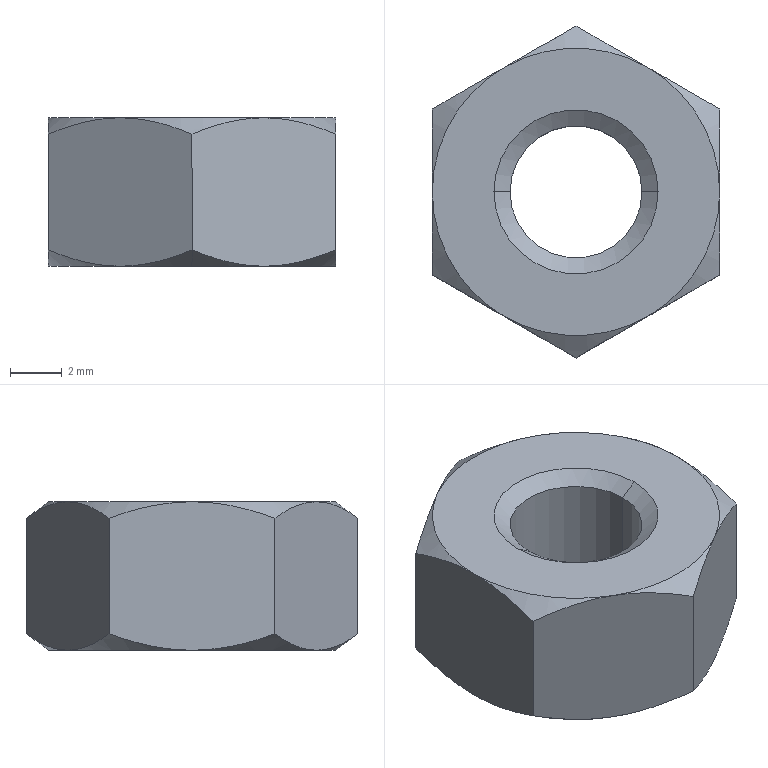Part | SolidWorks | features BaseBody 1 | 1 solid | 29 faces | box 11.113 x 12.832 x 5.74 mm | volume 487.574 mm3 | cone 17 | plane 8 | cylinder 4 | commonest cylinder face diameters 5.105 x2 6.35 x2
STEP:
#1=CARTESIAN_POINT('',(0.,-3.175,-5.74));
#2=VERTEX_POINT('',#1);
#3=CARTESIAN_POINT('',(0.,3.175,-5.74));
#4=VERTEX_POINT('',#3);
#5=CARTESIAN_POINT('',(0.,0.,-5.74));
#6=DIRECTION('',(0.,0.,-1.));
#7=DIRECTION('',(0.,-1.,0.));
#8=AXIS2_PLACEMENT_3D('',#5,#6,#7);
#9=CIRCLE('',#8,3.175);
#10=EDGE_CURVE('',#2,#4,#9,.T.);
#11=ORIENTED_EDGE('',*,*,#10,.T.);
#12=CARTESIAN_POINT('',(0.,3.175,-5.715));
#13=VERTEX_POINT('',#12);
#14=CARTESIAN_POINT('',(0.,3.175,-5.74));
#15=DIRECTION('',(0.,0.,1.));
#16=VECTOR('',#15,1000.);
#17=LINE('',#14,#16);
#18=EDGE_CURVE('',#4,#13,#17,.T.);
#19=ORIENTED_EDGE('',*,*,#18,.T.);
#20=CARTESIAN_POINT('',(-3.175,0.,-5.715));
#21=VERTEX_POINT('',#20);
#22=CARTESIAN_POINT('',(0.,0.,-5.715));
#23=DIRECTION('',(0.,0.,1.));
#24=DIRECTION('',(1.,0.,0.));
#25=AXIS2_PLACEMENT_3D('',#22,#23,#24);
#26=CIRCLE('',#25,3.175);
#27=EDGE_CURVE('',#13,#21,#26,.T.);
#28=ORIENTED_EDGE('',*,*,#27,.T.);
#29=CARTESIAN_POINT('',(0.,-3.175,-5.715));
#30=VERTEX_POINT('',#29);
#31=CARTESIAN_POINT('',(0.,0.,-5.715));
#32=DIRECTION('',(0.,0.,1.));
#33=DIRECTION('',(1.,0.,0.));
#34=AXIS2_PLACEMENT_3D('',#31,#32,#33);
#35=CIRCLE('',#34,3.175);
#36=EDGE_CURVE('',#21,#30,#35,.T.);
#37=ORIENTED_EDGE('',*,*,#36,.T.);
#38=CARTESIAN_POINT('',(0.,-3.175,-5.74));
#39=DIRECTION('',(0.,0.,1.));
#40=VECTOR('',#39,1000.);
#41=LINE('',#38,#40);
#42=EDGE_CURVE('',#2,#30,#41,.T.);
#43=ORIENTED_EDGE('',*,*,#42,.F.);
#44=EDGE_LOOP('',(#11,#19,#28,#37,#43));
#45=FACE_OUTER_BOUND('',#44,.T.);
#46=CARTESIAN_POINT('',(0.,0.,-5.74));
#47=DIRECTION('',(0.,0.,1.));
#48=DIRECTION('',(0.,-1.,0.));
#49=AXIS2_PLACEMENT_3D('',#46,#47,#48);
#50=CYLINDRICAL_SURFACE('',#49,3.175);
#51=ADVANCED_FACE('',(#45),#50,.F.);
#52=CARTESIAN_POINT('',(-2.553,0.,-5.279));
#53=VERTEX_POINT('',#52);
#54=CARTESIAN_POINT('',(2.553,0.,-5.279));
#55=VERTEX_POINT('',#54);
#56=CARTESIAN_POINT('',(0.,0.,-5.279));
#57=DIRECTION('',(0.,0.,1.));
#58=DIRECTION('',(-1.,0.,0.));
#59=AXIS2_PLACEMENT_3D('',#56,#57,#58);
#60=CIRCLE('',#59,2.553);
#61=EDGE_CURVE('',#53,#55,#60,.T.);
#62=ORIENTED_EDGE('',*,*,#61,.T.);
#63=CARTESIAN_POINT('',(3.175,0.,-5.715));
#64=VERTEX_POINT('',#63);
#65=CARTESIAN_POINT('',(2.553,0.,-5.279));
#66=DIRECTION('',(0.8192,0.,-0.5736));
#67=VECTOR('',#66,1000.);
#68=LINE('',#65,#67);
#69=EDGE_CURVE('',#55,#64,#68,.T.);
#70=ORIENTED_EDGE('',*,*,#69,.T.);
#71=CARTESIAN_POINT('',(0.,0.,-5.715));
#72=DIRECTION('',(0.,0.,1.));
#73=DIRECTION('',(1.,0.,0.));
#74=AXIS2_PLACEMENT_3D('',#71,#72,#73);
#75=CIRCLE('',#74,3.175);
#76=EDGE_CURVE('',#30,#64,#75,.T.);
#77=ORIENTED_EDGE('',*,*,#76,.F.);
#78=ORIENTED_EDGE('',*,*,#36,.F.);
#79=CARTESIAN_POINT('',(-2.553,0.,-5.279));
#80=DIRECTION('',(-0.8192,0.,-0.5736));
#81=VECTOR('',#80,1000.);
#82=LINE('',#79,#81);
#83=EDGE_CURVE('',#53,#21,#82,.T.);
#84=ORIENTED_EDGE('',*,*,#83,.F.);
#85=EDGE_LOOP('',(#62,#70,#77,#78,#84));
#86=FACE_OUTER_BOUND('',#85,.T.);
#87=CARTESIAN_POINT('',(0.,0.,-5.279));
#88=DIRECTION('',(0.,0.,-1.));
#89=DIRECTION('',(-1.,0.,0.));
#90=AXIS2_PLACEMENT_3D('',#87,#88,#89);
#91=CONICAL_SURFACE('',#90,2.553,0.9599);
#92=ADVANCED_FACE('',(#86),#91,.F.);
#93=ORIENTED_EDGE('',*,*,#61,.F.);
#94=CARTESIAN_POINT('',(-2.553,0.,-0.4357));
#95=VERTEX_POINT('',#94);
#96=CARTESIAN_POINT('',(-2.553,0.,-5.279));
#97=DIRECTION('',(0.,0.,1.));
#98=VECTOR('',#97,1000.);
#99=LINE('',#96,#98);
#100=EDGE_CURVE('',#53,#95,#99,.T.);
#101=ORIENTED_EDGE('',*,*,#100,.T.);
#102=CARTESIAN_POINT('',(2.553,0.,-0.4357));
#103=VERTEX_POINT('',#102);
#104=CARTESIAN_POINT('',(0.,0.,-0.4357));
#105=DIRECTION('',(0.,0.,1.));
#106=DIRECTION('',(1.,0.,0.));
#107=AXIS2_PLACEMENT_3D('',#104,#105,#106);
#108=CIRCLE('',#107,2.553);
#109=EDGE_CURVE('',#95,#103,#108,.T.);
#110=ORIENTED_EDGE('',*,*,#109,.T.);
#111=CARTESIAN_POINT('',(2.553,0.,-5.279));
#112=DIRECTION('',(0.,0.,1.));
#113=VECTOR('',#112,1000.);
#114=LINE('',#111,#113);
#115=EDGE_CURVE('',#55,#103,#114,.T.);
#116=ORIENTED_EDGE('',*,*,#115,.F.);
#117=EDGE_LOOP('',(#93,#101,#110,#116));
#118=FACE_OUTER_BOUND('',#117,.T.);
#119=CARTESIAN_POINT('',(0.,0.,-5.279));
#120=DIRECTION('',(0.,0.,1.));
#121=DIRECTION('',(1.,0.,0.));
#122=AXIS2_PLACEMENT_3D('',#119,#120,#121);
#123=CYLINDRICAL_SURFACE('',#122,2.553);
#124=ADVANCED_FACE('',(#118),#123,.F.);
#125=CARTESIAN_POINT('',(0.,-5.556,-5.74));
#126=VERTEX_POINT('',#125);
#127=CARTESIAN_POINT('',(-2.778,-4.812,-5.74));
#128=VERTEX_POINT('',#127);
#129=CARTESIAN_POINT('',(0.,0.,-5.74));
#130=DIRECTION('',(0.,0.,-1.));
#131=DIRECTION('',(0.,-1.,0.));
#132=AXIS2_PLACEMENT_3D('',#129,#130,#131);
#133=CIRCLE('',#132,5.556);
#134=EDGE_CURVE('',#126,#128,#133,.T.);
#135=ORIENTED_EDGE('',*,*,#134,.F.);
#136=CARTESIAN_POINT('',(0.,-6.416,-5.105));
#137=VERTEX_POINT('',#136);
#138=CARTESIAN_POINT('',(0.,-5.556,-5.74));
#139=DIRECTION('',(0.,-0.8043,0.5942));
#140=VECTOR('',#139,1000.);
#141=LINE('',#138,#140);
#142=EDGE_CURVE('',#126,#137,#141,.T.);
#143=ORIENTED_EDGE('',*,*,#142,.T.);
#144=CARTESIAN_POINT('',(-2.778,-4.812,-5.74));
#145=CARTESIAN_POINT('',(-2.3,-5.088,-5.74));
#146=CARTESIAN_POINT('',(-1.83,-5.359,-5.679));
#147=CARTESIAN_POINT('',(-0.9045,-5.894,-5.457));
#148=CARTESIAN_POINT('',(-0.4474,-6.158,-5.296));
#149=CARTESIAN_POINT('',(0.,-6.416,-5.105));
#150=B_SPLINE_CURVE_WITH_KNOTS('',3,(#144,#145,#146,#147,#148,#149),.UNSPECIFIED.,.F.,.F.,(4,2,4),(0.,0.001636,0.003271),.UNSPECIFIED.);
#151=EDGE_CURVE('',#128,#137,#150,.T.);
#152=ORIENTED_EDGE('',*,*,#151,.F.);
#153=EDGE_LOOP('',(#135,#143,#152));
#154=FACE_OUTER_BOUND('',#153,.T.);
#155=CARTESIAN_POINT('',(0.,0.,-5.74));
#156=DIRECTION('',(0.,0.,1.));
#157=DIRECTION('',(0.,-1.,0.));
#158=AXIS2_PLACEMENT_3D('',#155,#156,#157);
#159=CONICAL_SURFACE('',#158,5.556,0.9345);
#160=ADVANCED_FACE('',(#154),#159,.T.);
#161=ORIENTED_EDGE('',*,*,#109,.F.);
#162=CARTESIAN_POINT('',(-3.175,0.,0.));
#163=VERTEX_POINT('',#162);
#164=CARTESIAN_POINT('',(-2.553,0.,-0.4357));
#165=DIRECTION('',(-0.8192,0.,0.5736));
#166=VECTOR('',#165,1000.);
#167=LINE('',#164,#166);
#168=EDGE_CURVE('',#95,#163,#167,.T.);
#169=ORIENTED_EDGE('',*,*,#168,.T.);
#170=CARTESIAN_POINT('',(3.175,0.,0.));
#171=VERTEX_POINT('',#170);
#172=CARTESIAN_POINT('',(0.,0.,0.));
#173=DIRECTION('',(0.,0.,1.));
#174=DIRECTION('',(1.,0.,0.));
#175=AXIS2_PLACEMENT_3D('',#172,#173,#174);
#176=CIRCLE('',#175,3.175);
#177=EDGE_CURVE('',#163,#171,#176,.T.);
#178=ORIENTED_EDGE('',*,*,#177,.T.);
#179=CARTESIAN_POINT('',(2.553,0.,-0.4357));
#180=DIRECTION('',(0.8192,0.,0.5736));
#181=VECTOR('',#180,1000.);
#182=LINE('',#179,#181);
#183=EDGE_CURVE('',#103,#171,#182,.T.);
#184=ORIENTED_EDGE('',*,*,#183,.F.);
#185=EDGE_LOOP('',(#161,#169,#178,#184));
#186=FACE_OUTER_BOUND('',#185,.T.);
#187=CARTESIAN_POINT('',(0.,0.,-0.4357));
#188=DIRECTION('',(0.,0.,1.));
#189=DIRECTION('',(1.,0.,0.));
#190=AXIS2_PLACEMENT_3D('',#187,#188,#189);
#191=CONICAL_SURFACE('',#190,2.553,0.9599);
#192=ADVANCED_FACE('',(#186),#191,.F.);
#193=ORIENTED_EDGE('',*,*,#18,.F.);
#194=CARTESIAN_POINT('',(0.,0.,-5.74));
#195=DIRECTION('',(0.,0.,-1.));
#196=DIRECTION('',(0.,-1.,0.));
#197=AXIS2_PLACEMENT_3D('',#194,#195,#196);
#198=CIRCLE('',#197,3.175);
#199=EDGE_CURVE('',#4,#2,#198,.T.);
#200=ORIENTED_EDGE('',*,*,#199,.T.);
#201=ORIENTED_EDGE('',*,*,#42,.T.);
#202=ORIENTED_EDGE('',*,*,#76,.T.);
#203=CARTESIAN_POINT('',(0.,0.,-5.715));
#204=DIRECTION('',(0.,0.,1.));
#205=DIRECTION('',(1.,0.,0.));
#206=AXIS2_PLACEMENT_3D('',#203,#204,#205);
#207=CIRCLE('',#206,3.175);
#208=EDGE_CURVE('',#64,#13,#207,.T.);
#209=ORIENTED_EDGE('',*,*,#208,.T.);
#210=EDGE_LOOP('',(#193,#200,#201,#202,#209));
#211=FACE_OUTER_BOUND('',#210,.T.);
#212=CARTESIAN_POINT('',(0.,0.,-5.74));
#213=DIRECTION('',(0.,0.,1.));
#214=DIRECTION('',(0.,-1.,0.));
#215=AXIS2_PLACEMENT_3D('',#212,#213,#214);
#216=CYLINDRICAL_SURFACE('',#215,3.175);
#217=ADVANCED_FACE('',(#211),#216,.F.);
#218=ORIENTED_EDGE('',*,*,#69,.F.);
#219=CARTESIAN_POINT('',(0.,0.,-5.279));
#220=DIRECTION('',(0.,0.,1.));
#221=DIRECTION('',(-1.,0.,0.));
#222=AXIS2_PLACEMENT_3D('',#219,#220,#221);
#223=CIRCLE('',#222,2.553);
#224=EDGE_CURVE('',#55,#53,#223,.T.);
#225=ORIENTED_EDGE('',*,*,#224,.T.);
#226=ORIENTED_EDGE('',*,*,#83,.T.);
#227=ORIENTED_EDGE('',*,*,#27,.F.);
#228=ORIENTED_EDGE('',*,*,#208,.F.);
#229=EDGE_LOOP('',(#218,#225,#226,#227,#228));
#230=FACE_OUTER_BOUND('',#229,.T.);
#231=CARTESIAN_POINT('',(0.,0.,-5.279));
#232=DIRECTION('',(0.,0.,-1.));
#233=DIRECTION('',(-1.,0.,0.));
#234=AXIS2_PLACEMENT_3D('',#231,#232,#233);
#235=CONICAL_SURFACE('',#234,2.553,0.9599);
#236=ADVANCED_FACE('',(#230),#235,.F.);
#237=ORIENTED_EDGE('',*,*,#10,.F.);
#238=ORIENTED_EDGE('',*,*,#199,.F.);
#239=EDGE_LOOP('',(#237,#238));
#240=FACE_BOUND('',#239,.T.);
#241=CARTESIAN_POINT('',(5.556,0.,-5.74));
#242=VERTEX_POINT('',#241);
#243=CARTESIAN_POINT('',(2.778,-4.812,-5.74));
#244=VERTEX_POINT('',#243);
#245=CARTESIAN_POINT('',(0.,0.,-5.74));
#246=DIRECTION('',(0.,0.,-1.));
#247=DIRECTION('',(0.,-1.,0.));
#248=AXIS2_PLACEMENT_3D('',#245,#246,#247);
#249=CIRCLE('',#248,5.556);
#250=EDGE_CURVE('',#242,#244,#249,.T.);
#251=ORIENTED_EDGE('',*,*,#250,.T.);
#252=CARTESIAN_POINT('',(0.,0.,-5.74));
#253=DIRECTION('',(0.,0.,-1.));
#254=DIRECTION('',(0.,-1.,0.));
#255=AXIS2_PLACEMENT_3D('',#252,#253,#254);
#256=CIRCLE('',#255,5.556);
#257=EDGE_CURVE('',#244,#126,#256,.T.);
#258=ORIENTED_EDGE('',*,*,#257,.T.);
#259=ORIENTED_EDGE('',*,*,#134,.T.);
#260=CARTESIAN_POINT('',(-5.556,-0.000000001,-5.74));
#261=VERTEX_POINT('',#260);
#262=CARTESIAN_POINT('',(0.,0.,-5.74));
#263=DIRECTION('',(0.,0.,-1.));
#264=DIRECTION('',(0.,-1.,0.));
#265=AXIS2_PLACEMENT_3D('',#262,#263,#264);
#266=CIRCLE('',#265,5.556);
#267=EDGE_CURVE('',#128,#261,#266,.T.);
#268=ORIENTED_EDGE('',*,*,#267,.T.);
#269=CARTESIAN_POINT('',(-2.778,4.812,-5.74));
#270=VERTEX_POINT('',#269);
#271=CARTESIAN_POINT('',(0.,0.,-5.74));
#272=DIRECTION('',(0.,0.,-1.));
#273=DIRECTION('',(0.,-1.,0.));
#274=AXIS2_PLACEMENT_3D('',#271,#272,#273);
#275=CIRCLE('',#274,5.556);
#276=EDGE_CURVE('',#261,#270,#275,.T.);
#277=ORIENTED_EDGE('',*,*,#276,.T.);
#278=CARTESIAN_POINT('',(2.778,4.812,-5.74));
#279=VERTEX_POINT('',#278);
#280=CARTESIAN_POINT('',(0.,0.,-5.74));
#281=DIRECTION('',(0.,0.,-1.));
#282=DIRECTION('',(0.,-1.,0.));
#283=AXIS2_PLACEMENT_3D('',#280,#281,#282);
#284=CIRCLE('',#283,5.556);
#285=EDGE_CURVE('',#270,#279,#284,.T.);
#286=ORIENTED_EDGE('',*,*,#285,.T.);
#287=CARTESIAN_POINT('',(0.,0.,-5.74));
#288=DIRECTION('',(0.,0.,-1.));
#289=DIRECTION('',(0.,-1.,0.));
#290=AXIS2_PLACEMENT_3D('',#287,#288,#289);
#291=CIRCLE('',#290,5.556);
#292=EDGE_CURVE('',#279,#242,#291,.T.);
#293=ORIENTED_EDGE('',*,*,#292,.T.);
#294=EDGE_LOOP('',(#251,#258,#259,#268,#277,#286,#293));
#295=FACE_OUTER_BOUND('',#294,.T.);
#296=CARTESIAN_POINT('',(5.623,-5.623,-5.74));
#297=DIRECTION('',(0.,0.,-1.));
#298=DIRECTION('',(-1.,0.,0.));
#299=AXIS2_PLACEMENT_3D('',#296,#297,#298);
#300=PLANE('',#299);
#301=ADVANCED_FACE('',(#240,#295),#300,.T.);
#302=ORIENTED_EDGE('',*,*,#100,.F.);
#303=ORIENTED_EDGE('',*,*,#224,.F.);
#304=ORIENTED_EDGE('',*,*,#115,.T.);
#305=CARTESIAN_POINT('',(0.,0.,-0.4357));
#306=DIRECTION('',(0.,0.,1.));
#307=DIRECTION('',(1.,0.,0.));
#308=AXIS2_PLACEMENT_3D('',#305,#306,#307);
#309=CIRCLE('',#308,2.553);
#310=EDGE_CURVE('',#103,#95,#309,.T.);
#311=ORIENTED_EDGE('',*,*,#310,.T.);
#312=EDGE_LOOP('',(#302,#303,#304,#311));
#313=FACE_OUTER_BOUND('',#312,.T.);
#314=CARTESIAN_POINT('',(0.,0.,-5.279));
#315=DIRECTION('',(0.,0.,1.));
#316=DIRECTION('',(1.,0.,0.));
#317=AXIS2_PLACEMENT_3D('',#314,#315,#316);
#318=CYLINDRICAL_SURFACE('',#317,2.553);
#319=ADVANCED_FACE('',(#313),#318,.F.);
#320=ORIENTED_EDGE('',*,*,#142,.F.);
#321=ORIENTED_EDGE('',*,*,#257,.F.);
#322=CARTESIAN_POINT('',(0.,-6.416,-5.105));
#323=CARTESIAN_POINT('',(0.8968,-5.898,-5.488));
#324=CARTESIAN_POINT('',(1.816,-5.367,-5.74));
#325=CARTESIAN_POINT('',(2.778,-4.812,-5.74));
#326=B_SPLINE_CURVE_WITH_KNOTS('',3,(#322,#323,#324,#325),.UNSPECIFIED.,.F.,.F.,(4,4),(0.,0.00327),.UNSPECIFIED.);
#327=EDGE_CURVE('',#137,#244,#326,.T.);
#328=ORIENTED_EDGE('',*,*,#327,.F.);
#329=EDGE_LOOP('',(#320,#321,#328));
#330=FACE_OUTER_BOUND('',#329,.T.);
#331=CARTESIAN_POINT('',(0.,0.,-5.74));
#332=DIRECTION('',(0.,0.,1.));
#333=DIRECTION('',(0.,-1.,0.));
#334=AXIS2_PLACEMENT_3D('',#331,#332,#333);
#335=CONICAL_SURFACE('',#334,5.556,0.9345);
#336=ADVANCED_FACE('',(#330),#335,.T.);
#337=ORIENTED_EDGE('',*,*,#250,.F.);
#338=CARTESIAN_POINT('',(5.556,-3.208,-5.105));
#339=VERTEX_POINT('',#338);
#340=CARTESIAN_POINT('',(5.556,-3.208,-5.105));
#341=CARTESIAN_POINT('',(5.556,-2.172,-5.488));
#342=CARTESIAN_POINT('',(5.556,-1.111,-5.74));
#343=CARTESIAN_POINT('',(5.556,0.,-5.74));
#344=B_SPLINE_CURVE_WITH_KNOTS('',3,(#340,#341,#342,#343),.UNSPECIFIED.,.F.,.F.,(4,4),(0.,0.00327),.UNSPECIFIED.);
#345=EDGE_CURVE('',#339,#242,#344,.T.);
#346=ORIENTED_EDGE('',*,*,#345,.F.);
#347=CARTESIAN_POINT('',(2.778,-4.812,-5.74));
#348=CARTESIAN_POINT('',(3.257,-4.536,-5.74));
#349=CARTESIAN_POINT('',(3.726,-4.264,-5.679));
#350=CARTESIAN_POINT('',(4.652,-3.73,-5.457));
#351=CARTESIAN_POINT('',(5.109,-3.466,-5.296));
#352=CARTESIAN_POINT('',(5.556,-3.208,-5.105));
#353=B_SPLINE_CURVE_WITH_KNOTS('',3,(#347,#348,#349,#350,#351,#352),.UNSPECIFIED.,.F.,.F.,(4,2,4),(0.,0.001636,0.003271),.UNSPECIFIED.);
#354=EDGE_CURVE('',#244,#339,#353,.T.);
#355=ORIENTED_EDGE('',*,*,#354,.F.);
#356=EDGE_LOOP('',(#337,#346,#355));
#357=FACE_OUTER_BOUND('',#356,.T.);
#358=CARTESIAN_POINT('',(0.,0.,-5.74));
#359=DIRECTION('',(0.,0.,1.));
#360=DIRECTION('',(0.,-1.,0.));
#361=AXIS2_PLACEMENT_3D('',#358,#359,#360);
#362=CONICAL_SURFACE('',#361,5.556,0.9345);
#363=ADVANCED_FACE('',(#357),#362,.T.);
#364=CARTESIAN_POINT('',(5.556,3.208,-5.105));
#365=VERTEX_POINT('',#364);
#366=CARTESIAN_POINT('',(5.556,0.,-5.74));
#367=CARTESIAN_POINT('',(5.556,0.5527,-5.74));
#368=CARTESIAN_POINT('',(5.556,1.095,-5.679));
#369=CARTESIAN_POINT('',(5.556,2.163,-5.457));
#370=CARTESIAN_POINT('',(5.556,2.691,-5.296));
#371=CARTESIAN_POINT('',(5.556,3.208,-5.105));
#372=B_SPLINE_CURVE_WITH_KNOTS('',3,(#366,#367,#368,#369,#370,#371),.UNSPECIFIED.,.F.,.F.,(4,2,4),(0.,0.001636,0.003271),.UNSPECIFIED.);
#373=EDGE_CURVE('',#242,#365,#372,.T.);
#374=ORIENTED_EDGE('',*,*,#373,.F.);
#375=ORIENTED_EDGE('',*,*,#292,.F.);
#376=CARTESIAN_POINT('',(5.556,3.208,-5.105));
#377=CARTESIAN_POINT('',(4.659,3.726,-5.488));
#378=CARTESIAN_POINT('',(3.74,4.256,-5.74));
#379=CARTESIAN_POINT('',(2.778,4.812,-5.74));
#380=B_SPLINE_CURVE_WITH_KNOTS('',3,(#376,#377,#378,#379),.UNSPECIFIED.,.F.,.F.,(4,4),(0.,0.00327),.UNSPECIFIED.);
#381=EDGE_CURVE('',#365,#279,#380,.T.);
#382=ORIENTED_EDGE('',*,*,#381,.F.);
#383=EDGE_LOOP('',(#374,#375,#382));
#384=FACE_OUTER_BOUND('',#383,.T.);
#385=CARTESIAN_POINT('',(0.,0.,-5.74));
#386=DIRECTION('',(0.,0.,1.));
#387=DIRECTION('',(0.,-1.,0.));
#388=AXIS2_PLACEMENT_3D('',#385,#386,#387);
#389=CONICAL_SURFACE('',#388,5.556,0.9345);
#390=ADVANCED_FACE('',(#384),#389,.T.);
#391=CARTESIAN_POINT('',(0.,6.416,-5.105));
#392=VERTEX_POINT('',#391);
#393=CARTESIAN_POINT('',(2.778,4.812,-5.74));
#394=CARTESIAN_POINT('',(2.3,5.088,-5.74));
#395=CARTESIAN_POINT('',(1.83,5.359,-5.679));
#396=CARTESIAN_POINT('',(0.9045,5.894,-5.457));
#397=CARTESIAN_POINT('',(0.4474,6.158,-5.296));
#398=CARTESIAN_POINT('',(0.,6.416,-5.105));
#399=B_SPLINE_CURVE_WITH_KNOTS('',3,(#393,#394,#395,#396,#397,#398),.UNSPECIFIED.,.F.,.F.,(4,2,4),(0.,0.001636,0.003271),.UNSPECIFIED.);
#400=EDGE_CURVE('',#279,#392,#399,.T.);
#401=ORIENTED_EDGE('',*,*,#400,.F.);
#402=ORIENTED_EDGE('',*,*,#285,.F.);
#403=CARTESIAN_POINT('',(0.,6.416,-5.105));
#404=CARTESIAN_POINT('',(-0.8968,5.898,-5.488));
#405=CARTESIAN_POINT('',(-1.816,5.367,-5.74));
#406=CARTESIAN_POINT('',(-2.778,4.812,-5.74));
#407=B_SPLINE_CURVE_WITH_KNOTS('',3,(#403,#404,#405,#406),.UNSPECIFIED.,.F.,.F.,(4,4),(0.,0.00327),.UNSPECIFIED.);
#408=EDGE_CURVE('',#392,#270,#407,.T.);
#409=ORIENTED_EDGE('',*,*,#408,.F.);
#410=EDGE_LOOP('',(#401,#402,#409));
#411=FACE_OUTER_BOUND('',#410,.T.);
#412=CARTESIAN_POINT('',(0.,0.,-5.74));
#413=DIRECTION('',(0.,0.,1.));
#414=DIRECTION('',(0.,-1.,0.));
#415=AXIS2_PLACEMENT_3D('',#412,#413,#414);
#416=CONICAL_SURFACE('',#415,5.556,0.9345);
#417=ADVANCED_FACE('',(#411),#416,.T.);
#418=ORIENTED_EDGE('',*,*,#276,.F.);
#419=CARTESIAN_POINT('',(-5.556,3.208,-5.105));
#420=VERTEX_POINT('',#419);
#421=CARTESIAN_POINT('',(-5.556,3.208,-5.105));
#422=CARTESIAN_POINT('',(-5.556,2.172,-5.488));
#423=CARTESIAN_POINT('',(-5.556,1.111,-5.74));
#424=CARTESIAN_POINT('',(-5.556,-0.000000001,-5.74));
#425=B_SPLINE_CURVE_WITH_KNOTS('',3,(#421,#422,#423,#424),.UNSPECIFIED.,.F.,.F.,(4,4),(0.,0.00327),.UNSPECIFIED.);
#426=EDGE_CURVE('',#420,#261,#425,.T.);
#427=ORIENTED_EDGE('',*,*,#426,.F.);
#428=CARTESIAN_POINT('',(-2.778,4.812,-5.74));
#429=CARTESIAN_POINT('',(-3.257,4.536,-5.74));
#430=CARTESIAN_POINT('',(-3.726,4.264,-5.679));
#431=CARTESIAN_POINT('',(-4.652,3.73,-5.457));
#432=CARTESIAN_POINT('',(-5.109,3.466,-5.296));
#433=CARTESIAN_POINT('',(-5.556,3.208,-5.105));
#434=B_SPLINE_CURVE_WITH_KNOTS('',3,(#428,#429,#430,#431,#432,#433),.UNSPECIFIED.,.F.,.F.,(4,2,4),(0.,0.001636,0.003271),.UNSPECIFIED.);
#435=EDGE_CURVE('',#270,#420,#434,.T.);
#436=ORIENTED_EDGE('',*,*,#435,.F.);
#437=EDGE_LOOP('',(#418,#427,#436));
#438=FACE_OUTER_BOUND('',#437,.T.);
#439=CARTESIAN_POINT('',(0.,0.,-5.74));
#440=DIRECTION('',(0.,0.,1.));
#441=DIRECTION('',(0.,-1.,0.));
#442=AXIS2_PLACEMENT_3D('',#439,#440,#441);
#443=CONICAL_SURFACE('',#442,5.556,0.9345);
#444=ADVANCED_FACE('',(#438),#443,.T.);
#445=CARTESIAN_POINT('',(-5.556,-3.208,-5.105));
#446=VERTEX_POINT('',#445);
#447=CARTESIAN_POINT('',(-5.556,-0.000000001,-5.74));
#448=CARTESIAN_POINT('',(-5.556,-0.5527,-5.74));
#449=CARTESIAN_POINT('',(-5.556,-1.095,-5.679));
#450=CARTESIAN_POINT('',(-5.556,-2.163,-5.457));
#451=CARTESIAN_POINT('',(-5.556,-2.691,-5.296));
#452=CARTESIAN_POINT('',(-5.556,-3.208,-5.105));
#453=B_SPLINE_CURVE_WITH_KNOTS('',3,(#447,#448,#449,#450,#451,#452),.UNSPECIFIED.,.F.,.F.,(4,2,4),(0.,0.001636,0.003271),.UNSPECIFIED.);
#454=EDGE_CURVE('',#261,#446,#453,.T.);
#455=ORIENTED_EDGE('',*,*,#454,.F.);
#456=ORIENTED_EDGE('',*,*,#267,.F.);
#457=CARTESIAN_POINT('',(-5.556,-3.208,-5.105));
#458=CARTESIAN_POINT('',(-4.659,-3.726,-5.488));
#459=CARTESIAN_POINT('',(-3.74,-4.256,-5.74));
#460=CARTESIAN_POINT('',(-2.778,-4.812,-5.74));
#461=B_SPLINE_CURVE_WITH_KNOTS('',3,(#457,#458,#459,#460),.UNSPECIFIED.,.F.,.F.,(4,4),(0.,0.00327),.UNSPECIFIED.);
#462=EDGE_CURVE('',#446,#128,#461,.T.);
#463=ORIENTED_EDGE('',*,*,#462,.F.);
#464=EDGE_LOOP('',(#455,#456,#463));
#465=FACE_OUTER_BOUND('',#464,.T.);
#466=CARTESIAN_POINT('',(0.,0.,-5.74));
#467=DIRECTION('',(0.,0.,1.));
#468=DIRECTION('',(0.,-1.,0.));
#469=AXIS2_PLACEMENT_3D('',#466,#467,#468);
#470=CONICAL_SURFACE('',#469,5.556,0.9345);
#471=ADVANCED_FACE('',(#465),#470,.T.);
#472=ORIENTED_EDGE('',*,*,#168,.F.);
#473=ORIENTED_EDGE('',*,*,#310,.F.);
#474=ORIENTED_EDGE('',*,*,#183,.T.);
#475=CARTESIAN_POINT('',(0.,0.,0.));
#476=DIRECTION('',(0.,0.,1.));
#477=DIRECTION('',(1.,0.,0.));
#478=AXIS2_PLACEMENT_3D('',#475,#476,#477);
#479=CIRCLE('',#478,3.175);
#480=EDGE_CURVE('',#171,#163,#479,.T.);
#481=ORIENTED_EDGE('',*,*,#480,.T.);
#482=EDGE_LOOP('',(#472,#473,#474,#481));
#483=FACE_OUTER_BOUND('',#482,.T.);
#484=CARTESIAN_POINT('',(0.,0.,-0.4357));
#485=DIRECTION('',(0.,0.,1.));
#486=DIRECTION('',(1.,0.,0.));
#487=AXIS2_PLACEMENT_3D('',#484,#485,#486);
#488=CONICAL_SURFACE('',#487,2.553,0.9599);
#489=ADVANCED_FACE('',(#483),#488,.F.);
#490=ORIENTED_EDGE('',*,*,#327,.T.);
#491=ORIENTED_EDGE('',*,*,#354,.T.);
#492=CARTESIAN_POINT('',(5.556,-3.208,-0.635));
#493=VERTEX_POINT('',#492);
#494=CARTESIAN_POINT('',(5.556,-3.208,-2.87));
#495=DIRECTION('',(0.,0.,1.));
#496=VECTOR('',#495,1000.);
#497=LINE('',#494,#496);
#498=EDGE_CURVE('',#339,#493,#497,.T.);
#499=ORIENTED_EDGE('',*,*,#498,.T.);
#500=CARTESIAN_POINT('',(2.778,-4.812,0.));
#501=VERTEX_POINT('',#500);
#502=CARTESIAN_POINT('',(5.556,-3.208,-0.635));
#503=CARTESIAN_POINT('',(4.659,-3.726,-0.2525));
#504=CARTESIAN_POINT('',(3.74,-4.256,0.));
#505=CARTESIAN_POINT('',(2.778,-4.812,0.));
#506=B_SPLINE_CURVE_WITH_KNOTS('',3,(#502,#503,#504,#505),.UNSPECIFIED.,.F.,.F.,(4,4),(0.,0.00327),.UNSPECIFIED.);
#507=EDGE_CURVE('',#493,#501,#506,.T.);
#508=ORIENTED_EDGE('',*,*,#507,.T.);
#509=CARTESIAN_POINT('',(0.,-6.416,-0.635));
#510=VERTEX_POINT('',#509);
#511=CARTESIAN_POINT('',(2.778,-4.812,0.));
#512=CARTESIAN_POINT('',(2.3,-5.088,0.));
#513=CARTESIAN_POINT('',(1.83,-5.359,-0.06178));
#514=CARTESIAN_POINT('',(0.9045,-5.894,-0.2839));
#515=CARTESIAN_POINT('',(0.4474,-6.158,-0.4442));
#516=CARTESIAN_POINT('',(0.,-6.416,-0.635));
#517=B_SPLINE_CURVE_WITH_KNOTS('',3,(#511,#512,#513,#514,#515,#516),.UNSPECIFIED.,.F.,.F.,(4,2,4),(0.,0.001636,0.003271),.UNSPECIFIED.);
#518=EDGE_CURVE('',#501,#510,#517,.T.);
#519=ORIENTED_EDGE('',*,*,#518,.T.);
#520=CARTESIAN_POINT('',(0.,-6.416,-2.87));
#521=DIRECTION('',(0.,0.,-1.));
#522=VECTOR('',#521,1000.);
#523=LINE('',#520,#522);
#524=EDGE_CURVE('',#510,#137,#523,.T.);
#525=ORIENTED_EDGE('',*,*,#524,.T.);
#526=EDGE_LOOP('',(#490,#491,#499,#508,#519,#525));
#527=FACE_OUTER_BOUND('',#526,.T.);
#528=CARTESIAN_POINT('',(0.,-6.416,-5.775));
#529=DIRECTION('',(0.5,-0.866,0.));
#530=DIRECTION('',(0.866,0.5,0.));
#531=AXIS2_PLACEMENT_3D('',#528,#529,#530);
#532=PLANE('',#531);
#533=ADVANCED_FACE('',(#527),#532,.T.);
#534=ORIENTED_EDGE('',*,*,#462,.T.);
#535=ORIENTED_EDGE('',*,*,#151,.T.);
#536=ORIENTED_EDGE('',*,*,#524,.F.);
#537=CARTESIAN_POINT('',(-2.778,-4.812,0.));
#538=VERTEX_POINT('',#537);
#539=CARTESIAN_POINT('',(0.,-6.416,-0.635));
#540=CARTESIAN_POINT('',(-0.8968,-5.898,-0.2525));
#541=CARTESIAN_POINT('',(-1.816,-5.367,0.));
#542=CARTESIAN_POINT('',(-2.778,-4.812,0.));
#543=B_SPLINE_CURVE_WITH_KNOTS('',3,(#539,#540,#541,#542),.UNSPECIFIED.,.F.,.F.,(4,4),(0.,0.00327),.UNSPECIFIED.);
#544=EDGE_CURVE('',#510,#538,#543,.T.);
#545=ORIENTED_EDGE('',*,*,#544,.T.);
#546=CARTESIAN_POINT('',(-5.556,-3.208,-0.635));
#547=VERTEX_POINT('',#546);
#548=CARTESIAN_POINT('',(-2.778,-4.812,0.));
#549=CARTESIAN_POINT('',(-3.257,-4.536,0.));
#550=CARTESIAN_POINT('',(-3.726,-4.264,-0.06178));
#551=CARTESIAN_POINT('',(-4.652,-3.73,-0.2839));
#552=CARTESIAN_POINT('',(-5.109,-3.466,-0.4442));
#553=CARTESIAN_POINT('',(-5.556,-3.208,-0.635));
#554=B_SPLINE_CURVE_WITH_KNOTS('',3,(#548,#549,#550,#551,#552,#553),.UNSPECIFIED.,.F.,.F.,(4,2,4),(0.,0.001636,0.003271),.UNSPECIFIED.);
#555=EDGE_CURVE('',#538,#547,#554,.T.);
#556=ORIENTED_EDGE('',*,*,#555,.T.);
#557=CARTESIAN_POINT('',(-5.556,-3.208,-2.87));
#558=DIRECTION('',(0.,0.,-1.));
#559=VECTOR('',#558,1000.);
#560=LINE('',#557,#559);
#561=EDGE_CURVE('',#547,#446,#560,.T.);
#562=ORIENTED_EDGE('',*,*,#561,.T.);
#563=EDGE_LOOP('',(#534,#535,#536,#545,#556,#562));
#564=FACE_OUTER_BOUND('',#563,.T.);
#565=CARTESIAN_POINT('',(-5.556,-3.208,-5.775));
#566=DIRECTION('',(-0.5,-0.866,0.));
#567=DIRECTION('',(0.866,-0.5,0.));
#568=AXIS2_PLACEMENT_3D('',#565,#566,#567);
#569=PLANE('',#568);
#570=ADVANCED_FACE('',(#564),#569,.T.);
#571=ORIENTED_EDGE('',*,*,#498,.F.);
#572=ORIENTED_EDGE('',*,*,#345,.T.);
#573=ORIENTED_EDGE('',*,*,#373,.T.);
#574=CARTESIAN_POINT('',(5.556,3.208,-0.635));
#575=VERTEX_POINT('',#574);
#576=CARTESIAN_POINT('',(5.556,3.208,-2.87));
#577=DIRECTION('',(0.,0.,-1.));
#578=VECTOR('',#577,1000.);
#579=LINE('',#576,#578);
#580=EDGE_CURVE('',#575,#365,#579,.T.);
#581=ORIENTED_EDGE('',*,*,#580,.F.);
#582=CARTESIAN_POINT('',(5.556,-0.000000001,0.));
#583=VERTEX_POINT('',#582);
#584=CARTESIAN_POINT('',(5.556,-0.000000001,0.));
#585=CARTESIAN_POINT('',(5.556,0.5527,0.));
#586=CARTESIAN_POINT('',(5.556,1.095,-0.06178));
#587=CARTESIAN_POINT('',(5.556,2.163,-0.2839));
#588=CARTESIAN_POINT('',(5.556,2.691,-0.4442));
#589=CARTESIAN_POINT('',(5.556,3.208,-0.635));
#590=B_SPLINE_CURVE_WITH_KNOTS('',3,(#584,#585,#586,#587,#588,#589),.UNSPECIFIED.,.F.,.F.,(4,2,4),(0.,0.001636,0.003271),.UNSPECIFIED.);
#591=EDGE_CURVE('',#583,#575,#590,.T.);
#592=ORIENTED_EDGE('',*,*,#591,.F.);
#593=CARTESIAN_POINT('',(5.556,-3.208,-0.635));
#594=CARTESIAN_POINT('',(5.556,-2.172,-0.2525));
#595=CARTESIAN_POINT('',(5.556,-1.111,0.));
#596=CARTESIAN_POINT('',(5.556,-0.000000001,0.));
#597=B_SPLINE_CURVE_WITH_KNOTS('',3,(#593,#594,#595,#596),.UNSPECIFIED.,.F.,.F.,(4,4),(0.,0.00327),.UNSPECIFIED.);
#598=EDGE_CURVE('',#493,#583,#597,.T.);
#599=ORIENTED_EDGE('',*,*,#598,.F.);
#600=EDGE_LOOP('',(#571,#572,#573,#581,#592,#599));
#601=FACE_OUTER_BOUND('',#600,.T.);
#602=CARTESIAN_POINT('',(5.556,-3.208,-5.775));
#603=DIRECTION('',(-1.,0.,0.));
#604=DIRECTION('',(0.,0.,1.));
#605=AXIS2_PLACEMENT_3D('',#602,#603,#604);
#606=PLANE('',#605);
#607=ADVANCED_FACE('',(#601),#606,.F.);
#608=ORIENTED_EDGE('',*,*,#381,.T.);
#609=ORIENTED_EDGE('',*,*,#400,.T.);
#610=CARTESIAN_POINT('',(0.,6.416,-0.635));
#611=VERTEX_POINT('',#610);
#612=CARTESIAN_POINT('',(0.,6.416,-2.87));
#613=DIRECTION('',(0.,0.,1.));
#614=VECTOR('',#613,1000.);
#615=LINE('',#612,#614);
#616=EDGE_CURVE('',#392,#611,#615,.T.);
#617=ORIENTED_EDGE('',*,*,#616,.T.);
#618=CARTESIAN_POINT('',(2.778,4.812,0.));
#619=VERTEX_POINT('',#618);
#620=CARTESIAN_POINT('',(0.,6.416,-0.635));
#621=CARTESIAN_POINT('',(0.8968,5.898,-0.2525));
#622=CARTESIAN_POINT('',(1.816,5.367,0.));
#623=CARTESIAN_POINT('',(2.778,4.812,0.));
#624=B_SPLINE_CURVE_WITH_KNOTS('',3,(#620,#621,#622,#623),.UNSPECIFIED.,.F.,.F.,(4,4),(0.,0.00327),.UNSPECIFIED.);
#625=EDGE_CURVE('',#611,#619,#624,.T.);
#626=ORIENTED_EDGE('',*,*,#625,.T.);
#627=CARTESIAN_POINT('',(2.778,4.812,0.));
#628=CARTESIAN_POINT('',(3.257,4.536,0.));
#629=CARTESIAN_POINT('',(3.726,4.264,-0.06178));
#630=CARTESIAN_POINT('',(4.652,3.73,-0.2839));
#631=CARTESIAN_POINT('',(5.109,3.466,-0.4442));
#632=CARTESIAN_POINT('',(5.556,3.208,-0.635));
#633=B_SPLINE_CURVE_WITH_KNOTS('',3,(#627,#628,#629,#630,#631,#632),.UNSPECIFIED.,.F.,.F.,(4,2,4),(0.,0.001636,0.003271),.UNSPECIFIED.);
#634=EDGE_CURVE('',#619,#575,#633,.T.);
#635=ORIENTED_EDGE('',*,*,#634,.T.);
#636=ORIENTED_EDGE('',*,*,#580,.T.);
#637=EDGE_LOOP('',(#608,#609,#617,#626,#635,#636));
#638=FACE_OUTER_BOUND('',#637,.T.);
#639=CARTESIAN_POINT('',(5.556,3.208,-5.775));
#640=DIRECTION('',(0.5,0.866,0.));
#641=DIRECTION('',(-0.866,0.5,0.));
#642=AXIS2_PLACEMENT_3D('',#639,#640,#641);
#643=PLANE('',#642);
#644=ADVANCED_FACE('',(#638),#643,.T.);
#645=ORIENTED_EDGE('',*,*,#408,.T.);
#646=ORIENTED_EDGE('',*,*,#435,.T.);
#647=CARTESIAN_POINT('',(-5.556,3.208,-0.635));
#648=VERTEX_POINT('',#647);
#649=CARTESIAN_POINT('',(-5.556,3.208,-2.87));
#650=DIRECTION('',(0.,0.,1.));
#651=VECTOR('',#650,1000.);
#652=LINE('',#649,#651);
#653=EDGE_CURVE('',#420,#648,#652,.T.);
#654=ORIENTED_EDGE('',*,*,#653,.T.);
#655=CARTESIAN_POINT('',(-2.778,4.812,0.));
#656=VERTEX_POINT('',#655);
#657=CARTESIAN_POINT('',(-5.556,3.208,-0.635));
#658=CARTESIAN_POINT('',(-4.659,3.726,-0.2525));
#659=CARTESIAN_POINT('',(-3.74,4.256,0.));
#660=CARTESIAN_POINT('',(-2.778,4.812,0.));
#661=B_SPLINE_CURVE_WITH_KNOTS('',3,(#657,#658,#659,#660),.UNSPECIFIED.,.F.,.F.,(4,4),(0.,0.00327),.UNSPECIFIED.);
#662=EDGE_CURVE('',#648,#656,#661,.T.);
#663=ORIENTED_EDGE('',*,*,#662,.T.);
#664=CARTESIAN_POINT('',(-2.778,4.812,0.));
#665=CARTESIAN_POINT('',(-2.3,5.088,0.));
#666=CARTESIAN_POINT('',(-1.83,5.359,-0.06178));
#667=CARTESIAN_POINT('',(-0.9045,5.894,-0.2839));
#668=CARTESIAN_POINT('',(-0.4474,6.158,-0.4442));
#669=CARTESIAN_POINT('',(0.,6.416,-0.635));
#670=B_SPLINE_CURVE_WITH_KNOTS('',3,(#664,#665,#666,#667,#668,#669),.UNSPECIFIED.,.F.,.F.,(4,2,4),(0.,0.001636,0.003271),.UNSPECIFIED.);
#671=EDGE_CURVE('',#656,#611,#670,.T.);
#672=ORIENTED_EDGE('',*,*,#671,.T.);
#673=ORIENTED_EDGE('',*,*,#616,.F.);
#674=EDGE_LOOP('',(#645,#646,#654,#663,#672,#673));
#675=FACE_OUTER_BOUND('',#674,.T.);
#676=CARTESIAN_POINT('',(0.,6.416,-5.775));
#677=DIRECTION('',(-0.5,0.866,0.));
#678=DIRECTION('',(-0.866,-0.5,0.));
#679=AXIS2_PLACEMENT_3D('',#676,#677,#678);
#680=PLANE('',#679);
#681=ADVANCED_FACE('',(#675),#680,.T.);
#682=ORIENTED_EDGE('',*,*,#426,.T.);
#683=ORIENTED_EDGE('',*,*,#454,.T.);
#684=ORIENTED_EDGE('',*,*,#561,.F.);
#685=CARTESIAN_POINT('',(-5.556,0.,0.));
#686=VERTEX_POINT('',#685);
#687=CARTESIAN_POINT('',(-5.556,-3.208,-0.635));
#688=CARTESIAN_POINT('',(-5.556,-2.172,-0.2525));
#689=CARTESIAN_POINT('',(-5.556,-1.111,0.));
#690=CARTESIAN_POINT('',(-5.556,0.,0.));
#691=B_SPLINE_CURVE_WITH_KNOTS('',3,(#687,#688,#689,#690),.UNSPECIFIED.,.F.,.F.,(4,4),(0.,0.00327),.UNSPECIFIED.);
#692=EDGE_CURVE('',#547,#686,#691,.T.);
#693=ORIENTED_EDGE('',*,*,#692,.T.);
#694=CARTESIAN_POINT('',(-5.556,0.,0.));
#695=CARTESIAN_POINT('',(-5.556,0.5527,0.));
#696=CARTESIAN_POINT('',(-5.556,1.095,-0.06178));
#697=CARTESIAN_POINT('',(-5.556,2.163,-0.2839));
#698=CARTESIAN_POINT('',(-5.556,2.691,-0.4442));
#699=CARTESIAN_POINT('',(-5.556,3.208,-0.635));
#700=B_SPLINE_CURVE_WITH_KNOTS('',3,(#694,#695,#696,#697,#698,#699),.UNSPECIFIED.,.F.,.F.,(4,2,4),(0.,0.001636,0.003271),.UNSPECIFIED.);
#701=EDGE_CURVE('',#686,#648,#700,.T.);
#702=ORIENTED_EDGE('',*,*,#701,.T.);
#703=ORIENTED_EDGE('',*,*,#653,.F.);
#704=EDGE_LOOP('',(#682,#683,#684,#693,#702,#703));
#705=FACE_OUTER_BOUND('',#704,.T.);
#706=CARTESIAN_POINT('',(-5.556,-3.208,-5.775));
#707=DIRECTION('',(-1.,0.,0.));
#708=DIRECTION('',(0.,0.,1.));
#709=AXIS2_PLACEMENT_3D('',#706,#707,#708);
#710=PLANE('',#709);
#711=ADVANCED_FACE('',(#705),#710,.T.);
#712=ORIENTED_EDGE('',*,*,#480,.F.);
#713=ORIENTED_EDGE('',*,*,#177,.F.);
#714=EDGE_LOOP('',(#712,#713));
#715=FACE_BOUND('',#714,.T.);
#716=CARTESIAN_POINT('',(0.,0.,0.));
#717=DIRECTION('',(0.,0.,-1.));
#718=DIRECTION('',(-1.,0.,0.));
#719=AXIS2_PLACEMENT_3D('',#716,#717,#718);
#720=CIRCLE('',#719,5.556);
#721=EDGE_CURVE('',#538,#686,#720,.T.);
#722=ORIENTED_EDGE('',*,*,#721,.F.);
#723=CARTESIAN_POINT('',(0.,0.,0.));
#724=DIRECTION('',(0.,0.,-1.));
#725=DIRECTION('',(-1.,0.,0.));
#726=AXIS2_PLACEMENT_3D('',#723,#724,#725);
#727=CIRCLE('',#726,5.556);
#728=EDGE_CURVE('',#501,#538,#727,.T.);
#729=ORIENTED_EDGE('',*,*,#728,.F.);
#730=CARTESIAN_POINT('',(0.,0.,0.));
#731=DIRECTION('',(0.,0.,-1.));
#732=DIRECTION('',(-1.,0.,0.));
#733=AXIS2_PLACEMENT_3D('',#730,#731,#732);
#734=CIRCLE('',#733,5.556);
#735=EDGE_CURVE('',#583,#501,#734,.T.);
#736=ORIENTED_EDGE('',*,*,#735,.F.);
#737=CARTESIAN_POINT('',(0.,0.,0.));
#738=DIRECTION('',(0.,0.,-1.));
#739=DIRECTION('',(-1.,0.,0.));
#740=AXIS2_PLACEMENT_3D('',#737,#738,#739);
#741=CIRCLE('',#740,5.556);
#742=EDGE_CURVE('',#619,#583,#741,.T.);
#743=ORIENTED_EDGE('',*,*,#742,.F.);
#744=CARTESIAN_POINT('',(0.,0.,0.));
#745=DIRECTION('',(0.,0.,-1.));
#746=DIRECTION('',(-1.,0.,0.));
#747=AXIS2_PLACEMENT_3D('',#744,#745,#746);
#748=CIRCLE('',#747,5.556);
#749=EDGE_CURVE('',#656,#619,#748,.T.);
#750=ORIENTED_EDGE('',*,*,#749,.F.);
#751=CARTESIAN_POINT('',(0.,0.,0.));
#752=DIRECTION('',(0.,0.,-1.));
#753=DIRECTION('',(-1.,0.,0.));
#754=AXIS2_PLACEMENT_3D('',#751,#752,#753);
#755=CIRCLE('',#754,5.556);
#756=EDGE_CURVE('',#686,#656,#755,.T.);
#757=ORIENTED_EDGE('',*,*,#756,.F.);
#758=EDGE_LOOP('',(#722,#729,#736,#743,#750,#757));
#759=FACE_OUTER_BOUND('',#758,.T.);
#760=CARTESIAN_POINT('',(5.623,-5.623,0.));
#761=DIRECTION('',(0.,0.,-1.));
#762=DIRECTION('',(-1.,0.,0.));
#763=AXIS2_PLACEMENT_3D('',#760,#761,#762);
#764=PLANE('',#763);
#765=ADVANCED_FACE('',(#715,#759),#764,.F.);
#766=ORIENTED_EDGE('',*,*,#544,.F.);
#767=ORIENTED_EDGE('',*,*,#518,.F.);
#768=ORIENTED_EDGE('',*,*,#728,.T.);
#769=EDGE_LOOP('',(#766,#767,#768));
#770=FACE_OUTER_BOUND('',#769,.T.);
#771=CARTESIAN_POINT('',(0.,0.,0.));
#772=DIRECTION('',(0.,0.,-1.));
#773=DIRECTION('',(-1.,0.,0.));
#774=AXIS2_PLACEMENT_3D('',#771,#772,#773);
#775=CONICAL_SURFACE('',#774,5.556,0.9345);
#776=ADVANCED_FACE('',(#770),#775,.T.);
#777=ORIENTED_EDGE('',*,*,#735,.T.);
#778=ORIENTED_EDGE('',*,*,#507,.F.);
#779=ORIENTED_EDGE('',*,*,#598,.T.);
#780=EDGE_LOOP('',(#777,#778,#779));
#781=FACE_OUTER_BOUND('',#780,.T.);
#782=CARTESIAN_POINT('',(0.,0.,0.));
#783=DIRECTION('',(0.,0.,-1.));
#784=DIRECTION('',(-1.,0.,0.));
#785=AXIS2_PLACEMENT_3D('',#782,#783,#784);
#786=CONICAL_SURFACE('',#785,5.556,0.9345);
#787=ADVANCED_FACE('',(#781),#786,.T.);
#788=ORIENTED_EDGE('',*,*,#692,.F.);
#789=ORIENTED_EDGE('',*,*,#555,.F.);
#790=ORIENTED_EDGE('',*,*,#721,.T.);
#791=EDGE_LOOP('',(#788,#789,#790));
#792=FACE_OUTER_BOUND('',#791,.T.);
#793=CARTESIAN_POINT('',(0.,0.,0.));
#794=DIRECTION('',(0.,0.,-1.));
#795=DIRECTION('',(-1.,0.,0.));
#796=AXIS2_PLACEMENT_3D('',#793,#794,#795);
#797=CONICAL_SURFACE('',#796,5.556,0.9345);
#798=ADVANCED_FACE('',(#792),#797,.T.);
#799=ORIENTED_EDGE('',*,*,#591,.T.);
#800=ORIENTED_EDGE('',*,*,#634,.F.);
#801=ORIENTED_EDGE('',*,*,#742,.T.);
#802=EDGE_LOOP('',(#799,#800,#801));
#803=FACE_OUTER_BOUND('',#802,.T.);
#804=CARTESIAN_POINT('',(0.,0.,0.));
#805=DIRECTION('',(0.,0.,-1.));
#806=DIRECTION('',(-1.,0.,0.));
#807=AXIS2_PLACEMENT_3D('',#804,#805,#806);
#808=CONICAL_SURFACE('',#807,5.556,0.9345);
#809=ADVANCED_FACE('',(#803),#808,.T.);
#810=ORIENTED_EDGE('',*,*,#625,.F.);
#811=ORIENTED_EDGE('',*,*,#671,.F.);
#812=ORIENTED_EDGE('',*,*,#749,.T.);
#813=EDGE_LOOP('',(#810,#811,#812));
#814=FACE_OUTER_BOUND('',#813,.T.);
#815=CARTESIAN_POINT('',(0.,0.,0.));
#816=DIRECTION('',(0.,0.,-1.));
#817=DIRECTION('',(-1.,0.,0.));
#818=AXIS2_PLACEMENT_3D('',#815,#816,#817);
#819=CONICAL_SURFACE('',#818,5.556,0.9345);
#820=ADVANCED_FACE('',(#814),#819,.T.);
#821=ORIENTED_EDGE('',*,*,#756,.T.);
#822=ORIENTED_EDGE('',*,*,#662,.F.);
#823=ORIENTED_EDGE('',*,*,#701,.F.);
#824=EDGE_LOOP('',(#821,#822,#823));
#825=FACE_OUTER_BOUND('',#824,.T.);
#826=CARTESIAN_POINT('',(0.,0.,0.));
#827=DIRECTION('',(0.,0.,-1.));
#828=DIRECTION('',(-1.,0.,0.));
#829=AXIS2_PLACEMENT_3D('',#826,#827,#828);
#830=CONICAL_SURFACE('',#829,5.556,0.9345);
#831=ADVANCED_FACE('',(#825),#830,.T.);
#832=CLOSED_SHELL('',(#51,#92,#124,#160,#192,#217,#236,#301,#319,#336,#363,#390,#417,#444,#471,#489,#533,#570,#607,#644,#681,#711,#765,#776,#787,#798,#809,#820,#831));
#833=MANIFOLD_SOLID_BREP('',#832);
#834=CARTESIAN_POINT('',(0.,0.,0.));
#835=DIRECTION('',(0.,0.,1.));
#836=DIRECTION('',(1.,0.,0.));
#837=AXIS2_PLACEMENT_3D('',#834,#835,#836);
#838=(LENGTH_UNIT()NAMED_UNIT(*)SI_UNIT(.MILLI.,.METRE.));
#839=UNCERTAINTY_MEASURE_WITH_UNIT(LENGTH_MEASURE(0.00001),#838,'','');
#840=(NAMED_UNIT(*)PLANE_ANGLE_UNIT()SI_UNIT($,.RADIAN.));
#841=(NAMED_UNIT(*)SI_UNIT($,.STERADIAN.)SOLID_ANGLE_UNIT());
#842=(GEOMETRIC_REPRESENTATION_CONTEXT(3)GLOBAL_UNCERTAINTY_ASSIGNED_CONTEXT((#839))GLOBAL_UNIT_ASSIGNED_CONTEXT((#838,#840,#841))REPRESENTATION_CONTEXT('',''));
#843=ADVANCED_BREP_SHAPE_REPRESENTATION('',(#833,#837),#842);